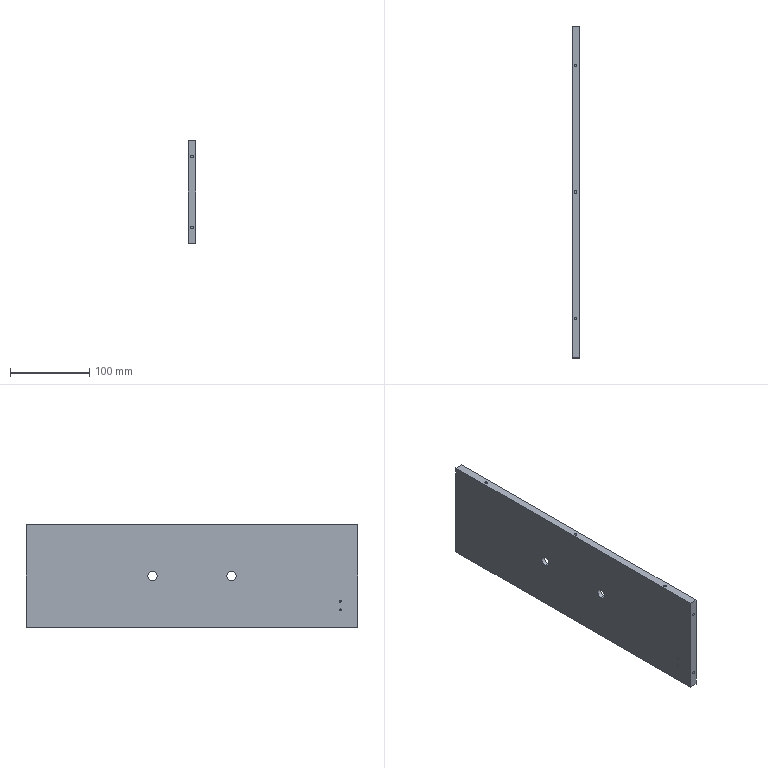Part | SolidWorks | features BaseBody 1 | 1 solid | 48 faces | box 10 x 420 x 130 mm | volume 527833 mm3 | cylinder 31 | plane 13 | cone 4 | commonest cylinder face diameters 3.3 x19 2.5 x4 12 x4 45 x4
STEP:
#1=CARTESIAN_POINT('',(-903.891,738.647,281.732));
#2=VERTEX_POINT('',#1);
#3=CARTESIAN_POINT('',(-905.541,740.297,281.732));
#4=VERTEX_POINT('',#3);
#5=CARTESIAN_POINT('',(-903.891,740.297,281.732));
#6=DIRECTION('',(0.,0.,-1.));
#7=DIRECTION('',(-1.,0.,0.));
#8=AXIS2_PLACEMENT_3D('',#5,#6,#7);
#9=CIRCLE('',#8,1.65);
#10=EDGE_CURVE('',#2,#4,#9,.T.);
#11=ORIENTED_EDGE('',*,*,#10,.T.);
#12=CARTESIAN_POINT('',(-905.541,740.297,301.732));
#13=VERTEX_POINT('',#12);
#14=CARTESIAN_POINT('',(-905.541,740.297,301.732));
#15=DIRECTION('',(0.,0.,1.));
#16=VECTOR('',#15,1000.);
#17=LINE('',#14,#16);
#18=EDGE_CURVE('',#4,#13,#17,.T.);
#19=ORIENTED_EDGE('',*,*,#18,.T.);
#20=CARTESIAN_POINT('',(-903.891,738.647,301.732));
#21=VERTEX_POINT('',#20);
#22=CARTESIAN_POINT('',(-903.891,740.297,301.732));
#23=DIRECTION('',(0.,0.,1.));
#24=DIRECTION('',(-1.,0.,0.));
#25=AXIS2_PLACEMENT_3D('',#22,#23,#24);
#26=CIRCLE('',#25,1.65);
#27=EDGE_CURVE('',#13,#21,#26,.T.);
#28=ORIENTED_EDGE('',*,*,#27,.T.);
#29=CARTESIAN_POINT('',(-903.891,738.647,301.732));
#30=DIRECTION('',(0.,0.,-1.));
#31=VECTOR('',#30,1000.);
#32=LINE('',#29,#31);
#33=EDGE_CURVE('',#21,#2,#32,.T.);
#34=ORIENTED_EDGE('',*,*,#33,.T.);
#35=EDGE_LOOP('',(#11,#19,#28,#34));
#36=FACE_OUTER_BOUND('',#35,.T.);
#37=CARTESIAN_POINT('',(-903.891,740.297,301.732));
#38=DIRECTION('',(0.,0.,1.));
#39=DIRECTION('',(-1.,0.,0.));
#40=AXIS2_PLACEMENT_3D('',#37,#38,#39);
#41=CYLINDRICAL_SURFACE('',#40,1.65);
#42=ADVANCED_FACE('',(#36),#41,.F.);
#43=CARTESIAN_POINT('',(-903.891,578.647,281.732));
#44=VERTEX_POINT('',#43);
#45=CARTESIAN_POINT('',(-905.541,580.297,281.732));
#46=VERTEX_POINT('',#45);
#47=CARTESIAN_POINT('',(-903.891,580.297,281.732));
#48=DIRECTION('',(0.,0.,-1.));
#49=DIRECTION('',(-1.,0.,0.));
#50=AXIS2_PLACEMENT_3D('',#47,#48,#49);
#51=CIRCLE('',#50,1.65);
#52=EDGE_CURVE('',#44,#46,#51,.T.);
#53=ORIENTED_EDGE('',*,*,#52,.T.);
#54=CARTESIAN_POINT('',(-905.541,580.297,301.732));
#55=VERTEX_POINT('',#54);
#56=CARTESIAN_POINT('',(-905.541,580.297,301.732));
#57=DIRECTION('',(0.,0.,1.));
#58=VECTOR('',#57,1000.);
#59=LINE('',#56,#58);
#60=EDGE_CURVE('',#46,#55,#59,.T.);
#61=ORIENTED_EDGE('',*,*,#60,.T.);
#62=CARTESIAN_POINT('',(-903.891,578.647,301.732));
#63=VERTEX_POINT('',#62);
#64=CARTESIAN_POINT('',(-903.891,580.297,301.732));
#65=DIRECTION('',(0.,0.,1.));
#66=DIRECTION('',(-1.,0.,0.));
#67=AXIS2_PLACEMENT_3D('',#64,#65,#66);
#68=CIRCLE('',#67,1.65);
#69=EDGE_CURVE('',#55,#63,#68,.T.);
#70=ORIENTED_EDGE('',*,*,#69,.T.);
#71=CARTESIAN_POINT('',(-903.891,578.647,301.732));
#72=DIRECTION('',(0.,0.,-1.));
#73=VECTOR('',#72,1000.);
#74=LINE('',#71,#73);
#75=EDGE_CURVE('',#63,#44,#74,.T.);
#76=ORIENTED_EDGE('',*,*,#75,.T.);
#77=EDGE_LOOP('',(#53,#61,#70,#76));
#78=FACE_OUTER_BOUND('',#77,.T.);
#79=CARTESIAN_POINT('',(-903.891,580.297,301.732));
#80=DIRECTION('',(0.,0.,1.));
#81=DIRECTION('',(-1.,0.,0.));
#82=AXIS2_PLACEMENT_3D('',#79,#80,#81);
#83=CYLINDRICAL_SURFACE('',#82,1.65);
#84=ADVANCED_FACE('',(#78),#83,.F.);
#85=CARTESIAN_POINT('',(-903.891,418.647,281.732));
#86=VERTEX_POINT('',#85);
#87=CARTESIAN_POINT('',(-905.541,420.297,281.732));
#88=VERTEX_POINT('',#87);
#89=CARTESIAN_POINT('',(-903.891,420.297,281.732));
#90=DIRECTION('',(0.,0.,-1.));
#91=DIRECTION('',(-1.,0.,0.));
#92=AXIS2_PLACEMENT_3D('',#89,#90,#91);
#93=CIRCLE('',#92,1.65);
#94=EDGE_CURVE('',#86,#88,#93,.T.);
#95=ORIENTED_EDGE('',*,*,#94,.T.);
#96=CARTESIAN_POINT('',(-905.541,420.297,301.732));
#97=VERTEX_POINT('',#96);
#98=CARTESIAN_POINT('',(-905.541,420.297,301.732));
#99=DIRECTION('',(0.,0.,1.));
#100=VECTOR('',#99,1000.);
#101=LINE('',#98,#100);
#102=EDGE_CURVE('',#88,#97,#101,.T.);
#103=ORIENTED_EDGE('',*,*,#102,.T.);
#104=CARTESIAN_POINT('',(-903.891,418.647,301.732));
#105=VERTEX_POINT('',#104);
#106=CARTESIAN_POINT('',(-903.891,420.297,301.732));
#107=DIRECTION('',(0.,0.,1.));
#108=DIRECTION('',(-1.,0.,0.));
#109=AXIS2_PLACEMENT_3D('',#106,#107,#108);
#110=CIRCLE('',#109,1.65);
#111=EDGE_CURVE('',#97,#105,#110,.T.);
#112=ORIENTED_EDGE('',*,*,#111,.T.);
#113=CARTESIAN_POINT('',(-903.891,418.647,301.732));
#114=DIRECTION('',(0.,0.,-1.));
#115=VECTOR('',#114,1000.);
#116=LINE('',#113,#115);
#117=EDGE_CURVE('',#105,#86,#116,.T.);
#118=ORIENTED_EDGE('',*,*,#117,.T.);
#119=EDGE_LOOP('',(#95,#103,#112,#118));
#120=FACE_OUTER_BOUND('',#119,.T.);
#121=CARTESIAN_POINT('',(-903.891,420.297,301.732));
#122=DIRECTION('',(0.,0.,1.));
#123=DIRECTION('',(-1.,0.,0.));
#124=AXIS2_PLACEMENT_3D('',#121,#122,#123);
#125=CYLINDRICAL_SURFACE('',#124,1.65);
#126=ADVANCED_FACE('',(#120),#125,.F.);
#127=CARTESIAN_POINT('',(-903.131,390.297,283.382));
#128=VERTEX_POINT('',#127);
#129=CARTESIAN_POINT('',(-901.481,390.297,281.732));
#130=VERTEX_POINT('',#129);
#131=CARTESIAN_POINT('',(-903.131,390.297,281.732));
#132=DIRECTION('',(0.,1.,0.));
#133=DIRECTION('',(1.,0.,0.));
#134=AXIS2_PLACEMENT_3D('',#131,#132,#133);
#135=CIRCLE('',#134,1.65);
#136=EDGE_CURVE('',#128,#130,#135,.T.);
#137=ORIENTED_EDGE('',*,*,#136,.T.);
#138=CARTESIAN_POINT('',(-901.481,370.297,281.732));
#139=VERTEX_POINT('',#138);
#140=CARTESIAN_POINT('',(-901.481,370.297,281.732));
#141=DIRECTION('',(0.,-1.,0.));
#142=VECTOR('',#141,1000.);
#143=LINE('',#140,#142);
#144=EDGE_CURVE('',#130,#139,#143,.T.);
#145=ORIENTED_EDGE('',*,*,#144,.T.);
#146=CARTESIAN_POINT('',(-903.131,370.297,283.382));
#147=VERTEX_POINT('',#146);
#148=CARTESIAN_POINT('',(-903.131,370.297,281.732));
#149=DIRECTION('',(0.,-1.,0.));
#150=DIRECTION('',(0.,0.,-1.));
#151=AXIS2_PLACEMENT_3D('',#148,#149,#150);
#152=CIRCLE('',#151,1.65);
#153=EDGE_CURVE('',#139,#147,#152,.T.);
#154=ORIENTED_EDGE('',*,*,#153,.T.);
#155=CARTESIAN_POINT('',(-903.131,390.297,283.382));
#156=DIRECTION('',(0.,-1.,0.));
#157=VECTOR('',#156,1000.);
#158=LINE('',#155,#157);
#159=EDGE_CURVE('',#128,#147,#158,.T.);
#160=ORIENTED_EDGE('',*,*,#159,.F.);
#161=EDGE_LOOP('',(#137,#145,#154,#160));
#162=FACE_OUTER_BOUND('',#161,.T.);
#163=CARTESIAN_POINT('',(-903.131,370.297,281.732));
#164=DIRECTION('',(0.,-1.,0.));
#165=DIRECTION('',(1.,0.,0.));
#166=AXIS2_PLACEMENT_3D('',#163,#164,#165);
#167=CYLINDRICAL_SURFACE('',#166,1.65);
#168=ADVANCED_FACE('',(#162),#167,.F.);
#169=CARTESIAN_POINT('',(-903.131,390.297,193.382));
#170=VERTEX_POINT('',#169);
#171=CARTESIAN_POINT('',(-901.481,390.297,191.732));
#172=VERTEX_POINT('',#171);
#173=CARTESIAN_POINT('',(-903.131,390.297,191.732));
#174=DIRECTION('',(0.,1.,0.));
#175=DIRECTION('',(1.,0.,0.));
#176=AXIS2_PLACEMENT_3D('',#173,#174,#175);
#177=CIRCLE('',#176,1.65);
#178=EDGE_CURVE('',#170,#172,#177,.T.);
#179=ORIENTED_EDGE('',*,*,#178,.T.);
#180=CARTESIAN_POINT('',(-901.481,370.297,191.732));
#181=VERTEX_POINT('',#180);
#182=CARTESIAN_POINT('',(-901.481,370.297,191.732));
#183=DIRECTION('',(0.,-1.,0.));
#184=VECTOR('',#183,1000.);
#185=LINE('',#182,#184);
#186=EDGE_CURVE('',#172,#181,#185,.T.);
#187=ORIENTED_EDGE('',*,*,#186,.T.);
#188=CARTESIAN_POINT('',(-903.131,370.297,193.382));
#189=VERTEX_POINT('',#188);
#190=CARTESIAN_POINT('',(-903.131,370.297,191.732));
#191=DIRECTION('',(0.,-1.,0.));
#192=DIRECTION('',(0.,0.,-1.));
#193=AXIS2_PLACEMENT_3D('',#190,#191,#192);
#194=CIRCLE('',#193,1.65);
#195=EDGE_CURVE('',#181,#189,#194,.T.);
#196=ORIENTED_EDGE('',*,*,#195,.T.);
#197=CARTESIAN_POINT('',(-903.131,390.297,193.382));
#198=DIRECTION('',(0.,-1.,0.));
#199=VECTOR('',#198,1000.);
#200=LINE('',#197,#199);
#201=EDGE_CURVE('',#170,#189,#200,.T.);
#202=ORIENTED_EDGE('',*,*,#201,.F.);
#203=EDGE_LOOP('',(#179,#187,#196,#202));
#204=FACE_OUTER_BOUND('',#203,.T.);
#205=CARTESIAN_POINT('',(-903.131,370.297,191.732));
#206=DIRECTION('',(0.,-1.,0.));
#207=DIRECTION('',(1.,0.,0.));
#208=AXIS2_PLACEMENT_3D('',#205,#206,#207);
#209=CYLINDRICAL_SURFACE('',#208,1.65);
#210=ADVANCED_FACE('',(#204),#209,.F.);
#211=CARTESIAN_POINT('',(-904.781,790.297,191.732));
#212=VERTEX_POINT('',#211);
#213=CARTESIAN_POINT('',(-901.481,790.297,191.732));
#214=VERTEX_POINT('',#213);
#215=CARTESIAN_POINT('',(-903.131,790.297,191.732));
#216=DIRECTION('',(0.,1.,0.));
#217=DIRECTION('',(-1.,0.,0.));
#218=AXIS2_PLACEMENT_3D('',#215,#216,#217);
#219=CIRCLE('',#218,1.65);
#220=EDGE_CURVE('',#212,#214,#219,.T.);
#221=ORIENTED_EDGE('',*,*,#220,.T.);
#222=CARTESIAN_POINT('',(-901.481,780.197,191.732));
#223=VERTEX_POINT('',#222);
#224=CARTESIAN_POINT('',(-901.481,780.197,191.732));
#225=DIRECTION('',(0.,1.,0.));
#226=VECTOR('',#225,1000.);
#227=LINE('',#224,#226);
#228=EDGE_CURVE('',#223,#214,#227,.T.);
#229=ORIENTED_EDGE('',*,*,#228,.F.);
#230=CARTESIAN_POINT('',(-904.781,780.197,191.732));
#231=VERTEX_POINT('',#230);
#232=CARTESIAN_POINT('',(-903.131,780.197,191.732));
#233=DIRECTION('',(0.,-1.,0.));
#234=DIRECTION('',(1.,0.,0.));
#235=AXIS2_PLACEMENT_3D('',#232,#233,#234);
#236=CIRCLE('',#235,1.65);
#237=EDGE_CURVE('',#223,#231,#236,.T.);
#238=ORIENTED_EDGE('',*,*,#237,.T.);
#239=CARTESIAN_POINT('',(-904.781,790.297,191.732));
#240=DIRECTION('',(0.,-1.,0.));
#241=VECTOR('',#240,1000.);
#242=LINE('',#239,#241);
#243=EDGE_CURVE('',#212,#231,#242,.T.);
#244=ORIENTED_EDGE('',*,*,#243,.F.);
#245=EDGE_LOOP('',(#221,#229,#238,#244));
#246=FACE_OUTER_BOUND('',#245,.T.);
#247=CARTESIAN_POINT('',(-903.131,790.297,191.732));
#248=DIRECTION('',(0.,1.,0.));
#249=DIRECTION('',(-1.,0.,0.));
#250=AXIS2_PLACEMENT_3D('',#247,#248,#249);
#251=CYLINDRICAL_SURFACE('',#250,1.65);
#252=ADVANCED_FACE('',(#246),#251,.F.);
#253=ORIENTED_EDGE('',*,*,#228,.T.);
#254=CARTESIAN_POINT('',(-903.131,790.297,191.732));
#255=DIRECTION('',(0.,1.,0.));
#256=DIRECTION('',(1.,0.,0.));
#257=AXIS2_PLACEMENT_3D('',#254,#255,#256);
#258=CIRCLE('',#257,1.65);
#259=EDGE_CURVE('',#214,#212,#258,.T.);
#260=ORIENTED_EDGE('',*,*,#259,.T.);
#261=ORIENTED_EDGE('',*,*,#243,.T.);
#262=CARTESIAN_POINT('',(-903.131,780.197,191.732));
#263=DIRECTION('',(0.,-1.,0.));
#264=DIRECTION('',(-1.,0.,0.));
#265=AXIS2_PLACEMENT_3D('',#262,#263,#264);
#266=CIRCLE('',#265,1.65);
#267=EDGE_CURVE('',#231,#223,#266,.T.);
#268=ORIENTED_EDGE('',*,*,#267,.T.);
#269=EDGE_LOOP('',(#253,#260,#261,#268));
#270=FACE_OUTER_BOUND('',#269,.T.);
#271=CARTESIAN_POINT('',(-903.131,790.297,191.732));
#272=DIRECTION('',(0.,1.,0.));
#273=DIRECTION('',(-1.,0.,0.));
#274=AXIS2_PLACEMENT_3D('',#271,#272,#273);
#275=CYLINDRICAL_SURFACE('',#274,1.65);
#276=ADVANCED_FACE('',(#270),#275,.F.);
#277=ORIENTED_EDGE('',*,*,#267,.F.);
#278=CARTESIAN_POINT('',(-903.131,779.205,191.732));
#279=VERTEX_POINT('',#278);
#280=CARTESIAN_POINT('',(-904.781,780.197,191.732));
#281=DIRECTION('',(0.8572,-0.515,0.));
#282=VECTOR('',#281,1000.);
#283=LINE('',#280,#282);
#284=EDGE_CURVE('',#231,#279,#283,.T.);
#285=ORIENTED_EDGE('',*,*,#284,.T.);
#286=CARTESIAN_POINT('',(-903.131,779.205,191.732));
#287=DIRECTION('',(0.8572,0.515,0.));
#288=VECTOR('',#287,1000.);
#289=LINE('',#286,#288);
#290=EDGE_CURVE('',#279,#223,#289,.T.);
#291=ORIENTED_EDGE('',*,*,#290,.T.);
#292=EDGE_LOOP('',(#277,#285,#291));
#293=FACE_OUTER_BOUND('',#292,.T.);
#294=CARTESIAN_POINT('',(-903.131,779.837,191.732));
#295=DIRECTION('',(0.,1.,0.));
#296=DIRECTION('',(1.,0.,0.));
#297=AXIS2_PLACEMENT_3D('',#294,#295,#296);
#298=CONICAL_SURFACE('',#297,1.051,1.03);
#299=ADVANCED_FACE('',(#293),#298,.F.);
#300=ORIENTED_EDGE('',*,*,#237,.F.);
#301=ORIENTED_EDGE('',*,*,#290,.F.);
#302=ORIENTED_EDGE('',*,*,#284,.F.);
#303=EDGE_LOOP('',(#300,#301,#302));
#304=FACE_OUTER_BOUND('',#303,.T.);
#305=CARTESIAN_POINT('',(-903.131,779.837,191.732));
#306=DIRECTION('',(0.,1.,0.));
#307=DIRECTION('',(1.,0.,0.));
#308=AXIS2_PLACEMENT_3D('',#305,#306,#307);
#309=CONICAL_SURFACE('',#308,1.051,1.03);
#310=ADVANCED_FACE('',(#304),#309,.F.);
#311=CARTESIAN_POINT('',(-898.131,790.297,171.732));
#312=VERTEX_POINT('',#311);
#313=CARTESIAN_POINT('',(-898.131,790.297,301.732));
#314=VERTEX_POINT('',#313);
#315=CARTESIAN_POINT('',(-898.131,790.297,171.732));
#316=DIRECTION('',(0.,0.,1.));
#317=VECTOR('',#316,1000.);
#318=LINE('',#315,#317);
#319=EDGE_CURVE('',#312,#314,#318,.T.);
#320=ORIENTED_EDGE('',*,*,#319,.F.);
#321=CARTESIAN_POINT('',(-908.131,790.297,171.732));
#322=VERTEX_POINT('',#321);
#323=CARTESIAN_POINT('',(-908.131,790.297,171.732));
#324=DIRECTION('',(1.,0.,0.));
#325=VECTOR('',#324,1000.);
#326=LINE('',#323,#325);
#327=EDGE_CURVE('',#322,#312,#326,.T.);
#328=ORIENTED_EDGE('',*,*,#327,.F.);
#329=CARTESIAN_POINT('',(-908.131,790.297,301.732));
#330=VERTEX_POINT('',#329);
#331=CARTESIAN_POINT('',(-908.131,790.297,301.732));
#332=DIRECTION('',(0.,0.,-1.));
#333=VECTOR('',#332,1000.);
#334=LINE('',#331,#333);
#335=EDGE_CURVE('',#330,#322,#334,.T.);
#336=ORIENTED_EDGE('',*,*,#335,.F.);
#337=CARTESIAN_POINT('',(-898.131,790.297,301.732));
#338=DIRECTION('',(-1.,0.,0.));
#339=VECTOR('',#338,1000.);
#340=LINE('',#337,#339);
#341=EDGE_CURVE('',#314,#330,#340,.T.);
#342=ORIENTED_EDGE('',*,*,#341,.F.);
#343=EDGE_LOOP('',(#320,#328,#336,#342));
#344=FACE_OUTER_BOUND('',#343,.T.);
#345=CARTESIAN_POINT('',(-901.481,790.297,281.732));
#346=VERTEX_POINT('',#345);
#347=CARTESIAN_POINT('',(-904.781,790.297,281.732));
#348=VERTEX_POINT('',#347);
#349=CARTESIAN_POINT('',(-903.131,790.297,281.732));
#350=DIRECTION('',(0.,1.,0.));
#351=DIRECTION('',(1.,0.,0.));
#352=AXIS2_PLACEMENT_3D('',#349,#350,#351);
#353=CIRCLE('',#352,1.65);
#354=EDGE_CURVE('',#346,#348,#353,.T.);
#355=ORIENTED_EDGE('',*,*,#354,.F.);
#356=CARTESIAN_POINT('',(-903.131,790.297,281.732));
#357=DIRECTION('',(0.,1.,0.));
#358=DIRECTION('',(-1.,0.,0.));
#359=AXIS2_PLACEMENT_3D('',#356,#357,#358);
#360=CIRCLE('',#359,1.65);
#361=EDGE_CURVE('',#348,#346,#360,.T.);
#362=ORIENTED_EDGE('',*,*,#361,.F.);
#363=EDGE_LOOP('',(#355,#362));
#364=FACE_BOUND('',#363,.T.);
#365=ORIENTED_EDGE('',*,*,#259,.F.);
#366=ORIENTED_EDGE('',*,*,#220,.F.);
#367=EDGE_LOOP('',(#365,#366));
#368=FACE_BOUND('',#367,.T.);
#369=CARTESIAN_POINT('',(-898.131,790.297,301.732));
#370=DIRECTION('',(0.,-1.,0.));
#371=DIRECTION('',(1.,0.,0.));
#372=AXIS2_PLACEMENT_3D('',#369,#370,#371);
#373=PLANE('',#372);
#374=ADVANCED_FACE('',(#344,#364,#368),#373,.F.);
#375=CARTESIAN_POINT('',(-898.131,370.297,301.732));
#376=VERTEX_POINT('',#375);
#377=CARTESIAN_POINT('',(-898.131,790.297,301.732));
#378=DIRECTION('',(0.,-1.,0.));
#379=VECTOR('',#378,1000.);
#380=LINE('',#377,#379);
#381=EDGE_CURVE('',#314,#376,#380,.T.);
#382=ORIENTED_EDGE('',*,*,#381,.F.);
#383=ORIENTED_EDGE('',*,*,#341,.T.);
#384=CARTESIAN_POINT('',(-908.131,370.297,301.732));
#385=VERTEX_POINT('',#384);
#386=CARTESIAN_POINT('',(-908.131,790.297,301.732));
#387=DIRECTION('',(0.,-1.,0.));
#388=VECTOR('',#387,1000.);
#389=LINE('',#386,#388);
#390=EDGE_CURVE('',#330,#385,#389,.T.);
#391=ORIENTED_EDGE('',*,*,#390,.T.);
#392=CARTESIAN_POINT('',(-908.131,370.297,301.732));
#393=DIRECTION('',(1.,0.,0.));
#394=VECTOR('',#393,1000.);
#395=LINE('',#392,#394);
#396=EDGE_CURVE('',#385,#376,#395,.T.);
#397=ORIENTED_EDGE('',*,*,#396,.T.);
#398=EDGE_LOOP('',(#382,#383,#391,#397));
#399=FACE_OUTER_BOUND('',#398,.T.);
#400=CARTESIAN_POINT('',(-903.891,421.947,301.732));
#401=VERTEX_POINT('',#400);
#402=CARTESIAN_POINT('',(-903.891,420.297,301.732));
#403=DIRECTION('',(0.,0.,1.));
#404=DIRECTION('',(-1.,0.,0.));
#405=AXIS2_PLACEMENT_3D('',#402,#403,#404);
#406=CIRCLE('',#405,1.65);
#407=EDGE_CURVE('',#401,#97,#406,.T.);
#408=ORIENTED_EDGE('',*,*,#407,.F.);
#409=CARTESIAN_POINT('',(-903.891,420.297,301.732));
#410=DIRECTION('',(0.,0.,1.));
#411=DIRECTION('',(0.,-1.,0.));
#412=AXIS2_PLACEMENT_3D('',#409,#410,#411);
#413=CIRCLE('',#412,1.65);
#414=EDGE_CURVE('',#105,#401,#413,.T.);
#415=ORIENTED_EDGE('',*,*,#414,.F.);
#416=ORIENTED_EDGE('',*,*,#111,.F.);
#417=EDGE_LOOP('',(#408,#415,#416));
#418=FACE_BOUND('',#417,.T.);
#419=CARTESIAN_POINT('',(-903.891,581.947,301.732));
#420=VERTEX_POINT('',#419);
#421=CARTESIAN_POINT('',(-903.891,580.297,301.732));
#422=DIRECTION('',(0.,0.,1.));
#423=DIRECTION('',(-1.,0.,0.));
#424=AXIS2_PLACEMENT_3D('',#421,#422,#423);
#425=CIRCLE('',#424,1.65);
#426=EDGE_CURVE('',#420,#55,#425,.T.);
#427=ORIENTED_EDGE('',*,*,#426,.F.);
#428=CARTESIAN_POINT('',(-903.891,580.297,301.732));
#429=DIRECTION('',(0.,0.,1.));
#430=DIRECTION('',(0.,-1.,0.));
#431=AXIS2_PLACEMENT_3D('',#428,#429,#430);
#432=CIRCLE('',#431,1.65);
#433=EDGE_CURVE('',#63,#420,#432,.T.);
#434=ORIENTED_EDGE('',*,*,#433,.F.);
#435=ORIENTED_EDGE('',*,*,#69,.F.);
#436=EDGE_LOOP('',(#427,#434,#435));
#437=FACE_BOUND('',#436,.T.);
#438=CARTESIAN_POINT('',(-903.891,741.947,301.732));
#439=VERTEX_POINT('',#438);
#440=CARTESIAN_POINT('',(-903.891,740.297,301.732));
#441=DIRECTION('',(0.,0.,1.));
#442=DIRECTION('',(-1.,0.,0.));
#443=AXIS2_PLACEMENT_3D('',#440,#441,#442);
#444=CIRCLE('',#443,1.65);
#445=EDGE_CURVE('',#439,#13,#444,.T.);
#446=ORIENTED_EDGE('',*,*,#445,.F.);
#447=CARTESIAN_POINT('',(-903.891,740.297,301.732));
#448=DIRECTION('',(0.,0.,1.));
#449=DIRECTION('',(0.,-1.,0.));
#450=AXIS2_PLACEMENT_3D('',#447,#448,#449);
#451=CIRCLE('',#450,1.65);
#452=EDGE_CURVE('',#21,#439,#451,.T.);
#453=ORIENTED_EDGE('',*,*,#452,.F.);
#454=ORIENTED_EDGE('',*,*,#27,.F.);
#455=EDGE_LOOP('',(#446,#453,#454));
#456=FACE_BOUND('',#455,.T.);
#457=CARTESIAN_POINT('',(-898.131,790.297,301.732));
#458=DIRECTION('',(0.,0.,-1.));
#459=DIRECTION('',(0.,-1.,0.));
#460=AXIS2_PLACEMENT_3D('',#457,#458,#459);
#461=PLANE('',#460);
#462=ADVANCED_FACE('',(#399,#418,#437,#456),#461,.F.);
#463=CARTESIAN_POINT('',(-898.131,370.297,171.732));
#464=VERTEX_POINT('',#463);
#465=CARTESIAN_POINT('',(-898.131,370.297,301.732));
#466=DIRECTION('',(0.,0.,-1.));
#467=VECTOR('',#466,1000.);
#468=LINE('',#465,#467);
#469=EDGE_CURVE('',#376,#464,#468,.T.);
#470=ORIENTED_EDGE('',*,*,#469,.F.);
#471=ORIENTED_EDGE('',*,*,#396,.F.);
#472=CARTESIAN_POINT('',(-908.131,370.297,171.732));
#473=VERTEX_POINT('',#472);
#474=CARTESIAN_POINT('',(-908.131,370.297,301.732));
#475=DIRECTION('',(0.,0.,-1.));
#476=VECTOR('',#475,1000.);
#477=LINE('',#474,#476);
#478=EDGE_CURVE('',#385,#473,#477,.T.);
#479=ORIENTED_EDGE('',*,*,#478,.T.);
#480=CARTESIAN_POINT('',(-908.131,370.297,171.732));
#481=DIRECTION('',(1.,0.,0.));
#482=VECTOR('',#481,1000.);
#483=LINE('',#480,#482);
#484=EDGE_CURVE('',#473,#464,#483,.T.);
#485=ORIENTED_EDGE('',*,*,#484,.T.);
#486=EDGE_LOOP('',(#470,#471,#479,#485));
#487=FACE_OUTER_BOUND('',#486,.T.);
#488=CARTESIAN_POINT('',(-903.131,370.297,190.082));
#489=VERTEX_POINT('',#488);
#490=CARTESIAN_POINT('',(-903.131,370.297,191.732));
#491=DIRECTION('',(0.,-1.,0.));
#492=DIRECTION('',(-1.,0.,0.));
#493=AXIS2_PLACEMENT_3D('',#490,#491,#492);
#494=CIRCLE('',#493,1.65);
#495=EDGE_CURVE('',#189,#489,#494,.T.);
#496=ORIENTED_EDGE('',*,*,#495,.F.);
#497=ORIENTED_EDGE('',*,*,#195,.F.);
#498=CARTESIAN_POINT('',(-903.131,370.297,191.732));
#499=DIRECTION('',(0.,-1.,0.));
#500=DIRECTION('',(0.,0.,-1.));
#501=AXIS2_PLACEMENT_3D('',#498,#499,#500);
#502=CIRCLE('',#501,1.65);
#503=EDGE_CURVE('',#489,#181,#502,.T.);
#504=ORIENTED_EDGE('',*,*,#503,.F.);
#505=EDGE_LOOP('',(#496,#497,#504));
#506=FACE_BOUND('',#505,.T.);
#507=CARTESIAN_POINT('',(-903.131,370.297,280.082));
#508=VERTEX_POINT('',#507);
#509=CARTESIAN_POINT('',(-903.131,370.297,281.732));
#510=DIRECTION('',(0.,-1.,0.));
#511=DIRECTION('',(-1.,0.,0.));
#512=AXIS2_PLACEMENT_3D('',#509,#510,#511);
#513=CIRCLE('',#512,1.65);
#514=EDGE_CURVE('',#147,#508,#513,.T.);
#515=ORIENTED_EDGE('',*,*,#514,.F.);
#516=ORIENTED_EDGE('',*,*,#153,.F.);
#517=CARTESIAN_POINT('',(-903.131,370.297,281.732));
#518=DIRECTION('',(0.,-1.,0.));
#519=DIRECTION('',(0.,0.,-1.));
#520=AXIS2_PLACEMENT_3D('',#517,#518,#519);
#521=CIRCLE('',#520,1.65);
#522=EDGE_CURVE('',#508,#139,#521,.T.);
#523=ORIENTED_EDGE('',*,*,#522,.F.);
#524=EDGE_LOOP('',(#515,#516,#523));
#525=FACE_BOUND('',#524,.T.);
#526=CARTESIAN_POINT('',(-898.131,370.297,301.732));
#527=DIRECTION('',(0.,1.,0.));
#528=DIRECTION('',(-1.,0.,0.));
#529=AXIS2_PLACEMENT_3D('',#526,#527,#528);
#530=PLANE('',#529);
#531=ADVANCED_FACE('',(#487,#506,#525),#530,.F.);
#532=CARTESIAN_POINT('',(-898.131,370.297,171.732));
#533=DIRECTION('',(0.,1.,0.));
#534=VECTOR('',#533,1000.);
#535=LINE('',#532,#534);
#536=EDGE_CURVE('',#464,#312,#535,.T.);
#537=ORIENTED_EDGE('',*,*,#536,.F.);
#538=ORIENTED_EDGE('',*,*,#484,.F.);
#539=CARTESIAN_POINT('',(-908.131,370.297,171.732));
#540=DIRECTION('',(0.,1.,0.));
#541=VECTOR('',#540,1000.);
#542=LINE('',#539,#541);
#543=EDGE_CURVE('',#473,#322,#542,.T.);
#544=ORIENTED_EDGE('',*,*,#543,.T.);
#545=ORIENTED_EDGE('',*,*,#327,.T.);
#546=EDGE_LOOP('',(#537,#538,#544,#545));
#547=FACE_OUTER_BOUND('',#546,.T.);
#548=CARTESIAN_POINT('',(-898.131,790.297,171.732));
#549=DIRECTION('',(0.,0.,1.));
#550=DIRECTION('',(0.,1.,0.));
#551=AXIS2_PLACEMENT_3D('',#548,#549,#550);
#552=PLANE('',#551);
#553=ADVANCED_FACE('',(#547),#552,.F.);
#554=ORIENTED_EDGE('',*,*,#390,.F.);
#555=ORIENTED_EDGE('',*,*,#335,.T.);
#556=ORIENTED_EDGE('',*,*,#543,.F.);
#557=ORIENTED_EDGE('',*,*,#478,.F.);
#558=EDGE_LOOP('',(#554,#555,#556,#557));
#559=FACE_OUTER_BOUND('',#558,.T.);
#560=CARTESIAN_POINT('',(-908.131,392.797,194.982));
#561=VERTEX_POINT('',#560);
#562=CARTESIAN_POINT('',(-908.131,392.797,192.482));
#563=VERTEX_POINT('',#562);
#564=CARTESIAN_POINT('',(-908.131,392.797,193.732));
#565=DIRECTION('',(-1.,0.,0.));
#566=DIRECTION('',(0.,0.,1.));
#567=AXIS2_PLACEMENT_3D('',#564,#565,#566);
#568=CIRCLE('',#567,1.25);
#569=EDGE_CURVE('',#561,#563,#568,.T.);
#570=ORIENTED_EDGE('',*,*,#569,.F.);
#571=CARTESIAN_POINT('',(-908.131,392.797,193.732));
#572=DIRECTION('',(-1.,0.,0.));
#573=DIRECTION('',(0.,0.,-1.));
#574=AXIS2_PLACEMENT_3D('',#571,#572,#573);
#575=CIRCLE('',#574,1.25);
#576=EDGE_CURVE('',#563,#561,#575,.T.);
#577=ORIENTED_EDGE('',*,*,#576,.F.);
#578=EDGE_LOOP('',(#570,#577));
#579=FACE_BOUND('',#578,.T.);
#580=CARTESIAN_POINT('',(-908.131,392.797,205.982));
#581=VERTEX_POINT('',#580);
#582=CARTESIAN_POINT('',(-908.131,392.797,203.482));
#583=VERTEX_POINT('',#582);
#584=CARTESIAN_POINT('',(-908.131,392.797,204.732));
#585=DIRECTION('',(-1.,0.,0.));
#586=DIRECTION('',(0.,0.,1.));
#587=AXIS2_PLACEMENT_3D('',#584,#585,#586);
#588=CIRCLE('',#587,1.25);
#589=EDGE_CURVE('',#581,#583,#588,.T.);
#590=ORIENTED_EDGE('',*,*,#589,.F.);
#591=CARTESIAN_POINT('',(-908.131,392.797,204.732));
#592=DIRECTION('',(-1.,0.,0.));
#593=DIRECTION('',(0.,0.,-1.));
#594=AXIS2_PLACEMENT_3D('',#591,#592,#593);
#595=CIRCLE('',#594,1.25);
#596=EDGE_CURVE('',#583,#581,#595,.T.);
#597=ORIENTED_EDGE('',*,*,#596,.F.);
#598=EDGE_LOOP('',(#590,#597));
#599=FACE_BOUND('',#598,.T.);
#600=CARTESIAN_POINT('',(-908.131,530.297,242.732));
#601=VERTEX_POINT('',#600);
#602=CARTESIAN_POINT('',(-908.131,530.297,230.732));
#603=VERTEX_POINT('',#602);
#604=CARTESIAN_POINT('',(-908.131,530.297,236.732));
#605=DIRECTION('',(-1.,0.,0.));
#606=DIRECTION('',(0.,0.,1.));
#607=AXIS2_PLACEMENT_3D('',#604,#605,#606);
#608=CIRCLE('',#607,6.);
#609=EDGE_CURVE('',#601,#603,#608,.T.);
#610=ORIENTED_EDGE('',*,*,#609,.F.);
#611=CARTESIAN_POINT('',(-908.131,530.297,236.732));
#612=DIRECTION('',(-1.,0.,0.));
#613=DIRECTION('',(0.,0.,-1.));
#614=AXIS2_PLACEMENT_3D('',#611,#612,#613);
#615=CIRCLE('',#614,6.);
#616=EDGE_CURVE('',#603,#601,#615,.T.);
#617=ORIENTED_EDGE('',*,*,#616,.F.);
#618=EDGE_LOOP('',(#610,#617));
#619=FACE_BOUND('',#618,.T.);
#620=CARTESIAN_POINT('',(-908.131,630.297,242.732));
#621=VERTEX_POINT('',#620);
#622=CARTESIAN_POINT('',(-908.131,630.297,230.732));
#623=VERTEX_POINT('',#622);
#624=CARTESIAN_POINT('',(-908.131,630.297,236.732));
#625=DIRECTION('',(-1.,0.,0.));
#626=DIRECTION('',(0.,0.,1.));
#627=AXIS2_PLACEMENT_3D('',#624,#625,#626);
#628=CIRCLE('',#627,6.);
#629=EDGE_CURVE('',#621,#623,#628,.T.);
#630=ORIENTED_EDGE('',*,*,#629,.F.);
#631=CARTESIAN_POINT('',(-908.131,630.297,236.732));
#632=DIRECTION('',(-1.,0.,0.));
#633=DIRECTION('',(0.,0.,-1.));
#634=AXIS2_PLACEMENT_3D('',#631,#632,#633);
#635=CIRCLE('',#634,6.);
#636=EDGE_CURVE('',#623,#621,#635,.T.);
#637=ORIENTED_EDGE('',*,*,#636,.F.);
#638=EDGE_LOOP('',(#630,#637));
#639=FACE_BOUND('',#638,.T.);
#640=CARTESIAN_POINT('',(-908.131,580.297,236.732));
#641=DIRECTION('',(1.,0.,0.));
#642=DIRECTION('',(0.,0.,1.));
#643=AXIS2_PLACEMENT_3D('',#640,#641,#642);
#644=PLANE('',#643);
#645=ADVANCED_FACE('',(#559,#579,#599,#619,#639),#644,.F.);
#646=ORIENTED_EDGE('',*,*,#576,.T.);
#647=CARTESIAN_POINT('',(-898.131,392.797,194.982));
#648=VERTEX_POINT('',#647);
#649=CARTESIAN_POINT('',(-898.131,392.797,194.982));
#650=DIRECTION('',(-1.,0.,0.));
#651=VECTOR('',#650,1000.);
#652=LINE('',#649,#651);
#653=EDGE_CURVE('',#648,#561,#652,.T.);
#654=ORIENTED_EDGE('',*,*,#653,.F.);
#655=CARTESIAN_POINT('',(-898.131,392.797,192.482));
#656=VERTEX_POINT('',#655);
#657=CARTESIAN_POINT('',(-898.131,392.797,193.732));
#658=DIRECTION('',(1.,0.,0.));
#659=DIRECTION('',(0.,0.,1.));
#660=AXIS2_PLACEMENT_3D('',#657,#658,#659);
#661=CIRCLE('',#660,1.25);
#662=EDGE_CURVE('',#648,#656,#661,.T.);
#663=ORIENTED_EDGE('',*,*,#662,.T.);
#664=CARTESIAN_POINT('',(-908.131,392.797,192.482));
#665=DIRECTION('',(1.,0.,0.));
#666=VECTOR('',#665,1000.);
#667=LINE('',#664,#666);
#668=EDGE_CURVE('',#563,#656,#667,.T.);
#669=ORIENTED_EDGE('',*,*,#668,.F.);
#670=EDGE_LOOP('',(#646,#654,#663,#669));
#671=FACE_OUTER_BOUND('',#670,.T.);
#672=CARTESIAN_POINT('',(-808.131,392.797,193.732));
#673=DIRECTION('',(-1.,0.,0.));
#674=DIRECTION('',(0.,0.,-1.));
#675=AXIS2_PLACEMENT_3D('',#672,#673,#674);
#676=CYLINDRICAL_SURFACE('',#675,1.25);
#677=ADVANCED_FACE('',(#671),#676,.F.);
#678=ORIENTED_EDGE('',*,*,#653,.T.);
#679=ORIENTED_EDGE('',*,*,#569,.T.);
#680=ORIENTED_EDGE('',*,*,#668,.T.);
#681=CARTESIAN_POINT('',(-898.131,392.797,193.732));
#682=DIRECTION('',(1.,0.,0.));
#683=DIRECTION('',(0.,0.,-1.));
#684=AXIS2_PLACEMENT_3D('',#681,#682,#683);
#685=CIRCLE('',#684,1.25);
#686=EDGE_CURVE('',#656,#648,#685,.T.);
#687=ORIENTED_EDGE('',*,*,#686,.T.);
#688=EDGE_LOOP('',(#678,#679,#680,#687));
#689=FACE_OUTER_BOUND('',#688,.T.);
#690=CARTESIAN_POINT('',(-808.131,392.797,193.732));
#691=DIRECTION('',(-1.,0.,0.));
#692=DIRECTION('',(0.,0.,-1.));
#693=AXIS2_PLACEMENT_3D('',#690,#691,#692);
#694=CYLINDRICAL_SURFACE('',#693,1.25);
#695=ADVANCED_FACE('',(#689),#694,.F.);
#696=ORIENTED_EDGE('',*,*,#381,.T.);
#697=ORIENTED_EDGE('',*,*,#469,.T.);
#698=ORIENTED_EDGE('',*,*,#536,.T.);
#699=ORIENTED_EDGE('',*,*,#319,.T.);
#700=EDGE_LOOP('',(#696,#697,#698,#699));
#701=FACE_OUTER_BOUND('',#700,.T.);
#702=ORIENTED_EDGE('',*,*,#662,.F.);
#703=ORIENTED_EDGE('',*,*,#686,.F.);
#704=EDGE_LOOP('',(#702,#703));
#705=FACE_BOUND('',#704,.T.);
#706=CARTESIAN_POINT('',(-898.131,392.797,205.982));
#707=VERTEX_POINT('',#706);
#708=CARTESIAN_POINT('',(-898.131,392.797,203.482));
#709=VERTEX_POINT('',#708);
#710=CARTESIAN_POINT('',(-898.131,392.797,204.732));
#711=DIRECTION('',(1.,0.,0.));
#712=DIRECTION('',(0.,0.,1.));
#713=AXIS2_PLACEMENT_3D('',#710,#711,#712);
#714=CIRCLE('',#713,1.25);
#715=EDGE_CURVE('',#707,#709,#714,.T.);
#716=ORIENTED_EDGE('',*,*,#715,.F.);
#717=CARTESIAN_POINT('',(-898.131,392.797,204.732));
#718=DIRECTION('',(1.,0.,0.));
#719=DIRECTION('',(0.,0.,-1.));
#720=AXIS2_PLACEMENT_3D('',#717,#718,#719);
#721=CIRCLE('',#720,1.25);
#722=EDGE_CURVE('',#709,#707,#721,.T.);
#723=ORIENTED_EDGE('',*,*,#722,.F.);
#724=EDGE_LOOP('',(#716,#723));
#725=FACE_BOUND('',#724,.T.);
#726=CARTESIAN_POINT('',(-898.131,530.297,214.232));
#727=VERTEX_POINT('',#726);
#728=CARTESIAN_POINT('',(-898.131,530.297,259.232));
#729=VERTEX_POINT('',#728);
#730=CARTESIAN_POINT('',(-898.131,530.297,236.732));
#731=DIRECTION('',(1.,0.,0.));
#732=DIRECTION('',(0.,0.,-1.));
#733=AXIS2_PLACEMENT_3D('',#730,#731,#732);
#734=CIRCLE('',#733,22.5);
#735=EDGE_CURVE('',#727,#729,#734,.T.);
#736=ORIENTED_EDGE('',*,*,#735,.F.);
#737=CARTESIAN_POINT('',(-898.131,530.297,236.732));
#738=DIRECTION('',(1.,0.,0.));
#739=DIRECTION('',(0.,0.,1.));
#740=AXIS2_PLACEMENT_3D('',#737,#738,#739);
#741=CIRCLE('',#740,22.5);
#742=EDGE_CURVE('',#729,#727,#741,.T.);
#743=ORIENTED_EDGE('',*,*,#742,.F.);
#744=EDGE_LOOP('',(#736,#743));
#745=FACE_BOUND('',#744,.T.);
#746=CARTESIAN_POINT('',(-898.131,630.297,214.232));
#747=VERTEX_POINT('',#746);
#748=CARTESIAN_POINT('',(-898.131,630.297,259.232));
#749=VERTEX_POINT('',#748);
#750=CARTESIAN_POINT('',(-898.131,630.297,236.732));
#751=DIRECTION('',(1.,0.,0.));
#752=DIRECTION('',(0.,0.,-1.));
#753=AXIS2_PLACEMENT_3D('',#750,#751,#752);
#754=CIRCLE('',#753,22.5);
#755=EDGE_CURVE('',#747,#749,#754,.T.);
#756=ORIENTED_EDGE('',*,*,#755,.F.);
#757=CARTESIAN_POINT('',(-898.131,630.297,236.732));
#758=DIRECTION('',(1.,0.,0.));
#759=DIRECTION('',(0.,0.,1.));
#760=AXIS2_PLACEMENT_3D('',#757,#758,#759);
#761=CIRCLE('',#760,22.5);
#762=EDGE_CURVE('',#749,#747,#761,.T.);
#763=ORIENTED_EDGE('',*,*,#762,.F.);
#764=EDGE_LOOP('',(#756,#763));
#765=FACE_BOUND('',#764,.T.);
#766=CARTESIAN_POINT('',(-898.131,580.297,236.732));
#767=DIRECTION('',(1.,0.,0.));
#768=DIRECTION('',(0.,0.,1.));
#769=AXIS2_PLACEMENT_3D('',#766,#767,#768);
#770=PLANE('',#769);
#771=ADVANCED_FACE('',(#701,#705,#725,#745,#765),#770,.T.);
#772=CARTESIAN_POINT('',(-898.131,392.797,205.982));
#773=DIRECTION('',(-1.,0.,0.));
#774=VECTOR('',#773,1000.);
#775=LINE('',#772,#774);
#776=EDGE_CURVE('',#707,#581,#775,.T.);
#777=ORIENTED_EDGE('',*,*,#776,.T.);
#778=ORIENTED_EDGE('',*,*,#589,.T.);
#779=CARTESIAN_POINT('',(-908.131,392.797,203.482));
#780=DIRECTION('',(1.,0.,0.));
#781=VECTOR('',#780,1000.);
#782=LINE('',#779,#781);
#783=EDGE_CURVE('',#583,#709,#782,.T.);
#784=ORIENTED_EDGE('',*,*,#783,.T.);
#785=ORIENTED_EDGE('',*,*,#722,.T.);
#786=EDGE_LOOP('',(#777,#778,#784,#785));
#787=FACE_OUTER_BOUND('',#786,.T.);
#788=CARTESIAN_POINT('',(-808.131,392.797,204.732));
#789=DIRECTION('',(-1.,0.,0.));
#790=DIRECTION('',(0.,0.,-1.));
#791=AXIS2_PLACEMENT_3D('',#788,#789,#790);
#792=CYLINDRICAL_SURFACE('',#791,1.25);
#793=ADVANCED_FACE('',(#787),#792,.F.);
#794=ORIENTED_EDGE('',*,*,#596,.T.);
#795=ORIENTED_EDGE('',*,*,#776,.F.);
#796=ORIENTED_EDGE('',*,*,#715,.T.);
#797=ORIENTED_EDGE('',*,*,#783,.F.);
#798=EDGE_LOOP('',(#794,#795,#796,#797));
#799=FACE_OUTER_BOUND('',#798,.T.);
#800=CARTESIAN_POINT('',(-808.131,392.797,204.732));
#801=DIRECTION('',(-1.,0.,0.));
#802=DIRECTION('',(0.,0.,-1.));
#803=AXIS2_PLACEMENT_3D('',#800,#801,#802);
#804=CYLINDRICAL_SURFACE('',#803,1.25);
#805=ADVANCED_FACE('',(#799),#804,.F.);
#806=ORIENTED_EDGE('',*,*,#742,.T.);
#807=CARTESIAN_POINT('',(-903.131,530.297,214.232));
#808=VERTEX_POINT('',#807);
#809=CARTESIAN_POINT('',(-898.131,530.297,214.232));
#810=DIRECTION('',(-1.,0.,0.));
#811=VECTOR('',#810,1000.);
#812=LINE('',#809,#811);
#813=EDGE_CURVE('',#727,#808,#812,.T.);
#814=ORIENTED_EDGE('',*,*,#813,.T.);
#815=CARTESIAN_POINT('',(-903.131,530.297,259.232));
#816=VERTEX_POINT('',#815);
#817=CARTESIAN_POINT('',(-903.131,530.297,236.732));
#818=DIRECTION('',(-1.,0.,0.));
#819=DIRECTION('',(0.,0.,-1.));
#820=AXIS2_PLACEMENT_3D('',#817,#818,#819);
#821=CIRCLE('',#820,22.5);
#822=EDGE_CURVE('',#808,#816,#821,.T.);
#823=ORIENTED_EDGE('',*,*,#822,.T.);
#824=CARTESIAN_POINT('',(-903.131,530.297,259.232));
#825=DIRECTION('',(1.,0.,0.));
#826=VECTOR('',#825,1000.);
#827=LINE('',#824,#826);
#828=EDGE_CURVE('',#816,#729,#827,.T.);
#829=ORIENTED_EDGE('',*,*,#828,.T.);
#830=EDGE_LOOP('',(#806,#814,#823,#829));
#831=FACE_OUTER_BOUND('',#830,.T.);
#832=CARTESIAN_POINT('',(-903.131,530.297,236.732));
#833=DIRECTION('',(1.,0.,0.));
#834=DIRECTION('',(0.,0.,1.));
#835=AXIS2_PLACEMENT_3D('',#832,#833,#834);
#836=CYLINDRICAL_SURFACE('',#835,22.5);
#837=ADVANCED_FACE('',(#831),#836,.F.);
#838=ORIENTED_EDGE('',*,*,#813,.F.);
#839=ORIENTED_EDGE('',*,*,#735,.T.);
#840=ORIENTED_EDGE('',*,*,#828,.F.);
#841=CARTESIAN_POINT('',(-903.131,530.297,236.732));
#842=DIRECTION('',(-1.,0.,0.));
#843=DIRECTION('',(0.,0.,1.));
#844=AXIS2_PLACEMENT_3D('',#841,#842,#843);
#845=CIRCLE('',#844,22.5);
#846=EDGE_CURVE('',#816,#808,#845,.T.);
#847=ORIENTED_EDGE('',*,*,#846,.T.);
#848=EDGE_LOOP('',(#838,#839,#840,#847));
#849=FACE_OUTER_BOUND('',#848,.T.);
#850=CARTESIAN_POINT('',(-903.131,530.297,236.732));
#851=DIRECTION('',(1.,0.,0.));
#852=DIRECTION('',(0.,0.,1.));
#853=AXIS2_PLACEMENT_3D('',#850,#851,#852);
#854=CYLINDRICAL_SURFACE('',#853,22.5);
#855=ADVANCED_FACE('',(#849),#854,.F.);
#856=ORIENTED_EDGE('',*,*,#846,.F.);
#857=ORIENTED_EDGE('',*,*,#822,.F.);
#858=EDGE_LOOP('',(#856,#857));
#859=FACE_OUTER_BOUND('',#858,.T.);
#860=CARTESIAN_POINT('',(-903.131,530.297,230.732));
#861=VERTEX_POINT('',#860);
#862=CARTESIAN_POINT('',(-903.131,530.297,242.732));
#863=VERTEX_POINT('',#862);
#864=CARTESIAN_POINT('',(-903.131,530.297,236.732));
#865=DIRECTION('',(1.,0.,0.));
#866=DIRECTION('',(0.,0.,-1.));
#867=AXIS2_PLACEMENT_3D('',#864,#865,#866);
#868=CIRCLE('',#867,6.);
#869=EDGE_CURVE('',#861,#863,#868,.T.);
#870=ORIENTED_EDGE('',*,*,#869,.F.);
#871=CARTESIAN_POINT('',(-903.131,530.297,236.732));
#872=DIRECTION('',(1.,0.,0.));
#873=DIRECTION('',(0.,0.,1.));
#874=AXIS2_PLACEMENT_3D('',#871,#872,#873);
#875=CIRCLE('',#874,6.);
#876=EDGE_CURVE('',#863,#861,#875,.T.);
#877=ORIENTED_EDGE('',*,*,#876,.F.);
#878=EDGE_LOOP('',(#870,#877));
#879=FACE_BOUND('',#878,.T.);
#880=CARTESIAN_POINT('',(-903.131,530.297,236.732));
#881=DIRECTION('',(1.,0.,0.));
#882=DIRECTION('',(0.,0.,1.));
#883=AXIS2_PLACEMENT_3D('',#880,#881,#882);
#884=PLANE('',#883);
#885=ADVANCED_FACE('',(#859,#879),#884,.T.);
#886=ORIENTED_EDGE('',*,*,#616,.T.);
#887=CARTESIAN_POINT('',(-908.131,530.297,242.732));
#888=DIRECTION('',(1.,0.,0.));
#889=VECTOR('',#888,1000.);
#890=LINE('',#887,#889);
#891=EDGE_CURVE('',#601,#863,#890,.T.);
#892=ORIENTED_EDGE('',*,*,#891,.T.);
#893=ORIENTED_EDGE('',*,*,#876,.T.);
#894=CARTESIAN_POINT('',(-903.131,530.297,230.732));
#895=DIRECTION('',(-1.,0.,0.));
#896=VECTOR('',#895,1000.);
#897=LINE('',#894,#896);
#898=EDGE_CURVE('',#861,#603,#897,.T.);
#899=ORIENTED_EDGE('',*,*,#898,.T.);
#900=EDGE_LOOP('',(#886,#892,#893,#899));
#901=FACE_OUTER_BOUND('',#900,.T.);
#902=CARTESIAN_POINT('',(-898.131,530.297,236.732));
#903=DIRECTION('',(-1.,0.,0.));
#904=DIRECTION('',(0.,0.,-1.));
#905=AXIS2_PLACEMENT_3D('',#902,#903,#904);
#906=CYLINDRICAL_SURFACE('',#905,6.);
#907=ADVANCED_FACE('',(#901),#906,.F.);
#908=ORIENTED_EDGE('',*,*,#891,.F.);
#909=ORIENTED_EDGE('',*,*,#609,.T.);
#910=ORIENTED_EDGE('',*,*,#898,.F.);
#911=ORIENTED_EDGE('',*,*,#869,.T.);
#912=EDGE_LOOP('',(#908,#909,#910,#911));
#913=FACE_OUTER_BOUND('',#912,.T.);
#914=CARTESIAN_POINT('',(-898.131,530.297,236.732));
#915=DIRECTION('',(-1.,0.,0.));
#916=DIRECTION('',(0.,0.,-1.));
#917=AXIS2_PLACEMENT_3D('',#914,#915,#916);
#918=CYLINDRICAL_SURFACE('',#917,6.);
#919=ADVANCED_FACE('',(#913),#918,.F.);
#920=ORIENTED_EDGE('',*,*,#762,.T.);
#921=CARTESIAN_POINT('',(-903.131,630.297,214.232));
#922=VERTEX_POINT('',#921);
#923=CARTESIAN_POINT('',(-898.131,630.297,214.232));
#924=DIRECTION('',(-1.,0.,0.));
#925=VECTOR('',#924,1000.);
#926=LINE('',#923,#925);
#927=EDGE_CURVE('',#747,#922,#926,.T.);
#928=ORIENTED_EDGE('',*,*,#927,.T.);
#929=CARTESIAN_POINT('',(-903.131,630.297,259.232));
#930=VERTEX_POINT('',#929);
#931=CARTESIAN_POINT('',(-903.131,630.297,236.732));
#932=DIRECTION('',(-1.,0.,0.));
#933=DIRECTION('',(0.,0.,-1.));
#934=AXIS2_PLACEMENT_3D('',#931,#932,#933);
#935=CIRCLE('',#934,22.5);
#936=EDGE_CURVE('',#922,#930,#935,.T.);
#937=ORIENTED_EDGE('',*,*,#936,.T.);
#938=CARTESIAN_POINT('',(-903.131,630.297,259.232));
#939=DIRECTION('',(1.,0.,0.));
#940=VECTOR('',#939,1000.);
#941=LINE('',#938,#940);
#942=EDGE_CURVE('',#930,#749,#941,.T.);
#943=ORIENTED_EDGE('',*,*,#942,.T.);
#944=EDGE_LOOP('',(#920,#928,#937,#943));
#945=FACE_OUTER_BOUND('',#944,.T.);
#946=CARTESIAN_POINT('',(-903.131,630.297,236.732));
#947=DIRECTION('',(1.,0.,0.));
#948=DIRECTION('',(0.,0.,1.));
#949=AXIS2_PLACEMENT_3D('',#946,#947,#948);
#950=CYLINDRICAL_SURFACE('',#949,22.5);
#951=ADVANCED_FACE('',(#945),#950,.F.);
#952=ORIENTED_EDGE('',*,*,#927,.F.);
#953=ORIENTED_EDGE('',*,*,#755,.T.);
#954=ORIENTED_EDGE('',*,*,#942,.F.);
#955=CARTESIAN_POINT('',(-903.131,630.297,236.732));
#956=DIRECTION('',(-1.,0.,0.));
#957=DIRECTION('',(0.,0.,1.));
#958=AXIS2_PLACEMENT_3D('',#955,#956,#957);
#959=CIRCLE('',#958,22.5);
#960=EDGE_CURVE('',#930,#922,#959,.T.);
#961=ORIENTED_EDGE('',*,*,#960,.T.);
#962=EDGE_LOOP('',(#952,#953,#954,#961));
#963=FACE_OUTER_BOUND('',#962,.T.);
#964=CARTESIAN_POINT('',(-903.131,630.297,236.732));
#965=DIRECTION('',(1.,0.,0.));
#966=DIRECTION('',(0.,0.,1.));
#967=AXIS2_PLACEMENT_3D('',#964,#965,#966);
#968=CYLINDRICAL_SURFACE('',#967,22.5);
#969=ADVANCED_FACE('',(#963),#968,.F.);
#970=ORIENTED_EDGE('',*,*,#960,.F.);
#971=ORIENTED_EDGE('',*,*,#936,.F.);
#972=EDGE_LOOP('',(#970,#971));
#973=FACE_OUTER_BOUND('',#972,.T.);
#974=CARTESIAN_POINT('',(-903.131,630.297,230.732));
#975=VERTEX_POINT('',#974);
#976=CARTESIAN_POINT('',(-903.131,630.297,242.732));
#977=VERTEX_POINT('',#976);
#978=CARTESIAN_POINT('',(-903.131,630.297,236.732));
#979=DIRECTION('',(1.,0.,0.));
#980=DIRECTION('',(0.,0.,-1.));
#981=AXIS2_PLACEMENT_3D('',#978,#979,#980);
#982=CIRCLE('',#981,6.);
#983=EDGE_CURVE('',#975,#977,#982,.T.);
#984=ORIENTED_EDGE('',*,*,#983,.F.);
#985=CARTESIAN_POINT('',(-903.131,630.297,236.732));
#986=DIRECTION('',(1.,0.,0.));
#987=DIRECTION('',(0.,0.,1.));
#988=AXIS2_PLACEMENT_3D('',#985,#986,#987);
#989=CIRCLE('',#988,6.);
#990=EDGE_CURVE('',#977,#975,#989,.T.);
#991=ORIENTED_EDGE('',*,*,#990,.F.);
#992=EDGE_LOOP('',(#984,#991));
#993=FACE_BOUND('',#992,.T.);
#994=CARTESIAN_POINT('',(-903.131,630.297,236.732));
#995=DIRECTION('',(1.,0.,0.));
#996=DIRECTION('',(0.,0.,1.));
#997=AXIS2_PLACEMENT_3D('',#994,#995,#996);
#998=PLANE('',#997);
#999=ADVANCED_FACE('',(#973,#993),#998,.T.);
#1000=ORIENTED_EDGE('',*,*,#636,.T.);
#1001=CARTESIAN_POINT('',(-908.131,630.297,242.732));
#1002=DIRECTION('',(1.,0.,0.));
#1003=VECTOR('',#1002,1000.);
#1004=LINE('',#1001,#1003);
#1005=EDGE_CURVE('',#621,#977,#1004,.T.);
#1006=ORIENTED_EDGE('',*,*,#1005,.T.);
#1007=ORIENTED_EDGE('',*,*,#990,.T.);
#1008=CARTESIAN_POINT('',(-903.131,630.297,230.732));
#1009=DIRECTION('',(-1.,0.,0.));
#1010=VECTOR('',#1009,1000.);
#1011=LINE('',#1008,#1010);
#1012=EDGE_CURVE('',#975,#623,#1011,.T.);
#1013=ORIENTED_EDGE('',*,*,#1012,.T.);
#1014=EDGE_LOOP('',(#1000,#1006,#1007,#1013));
#1015=FACE_OUTER_BOUND('',#1014,.T.);
#1016=CARTESIAN_POINT('',(-898.131,630.297,236.732));
#1017=DIRECTION('',(-1.,0.,0.));
#1018=DIRECTION('',(0.,0.,-1.));
#1019=AXIS2_PLACEMENT_3D('',#1016,#1017,#1018);
#1020=CYLINDRICAL_SURFACE('',#1019,6.);
#1021=ADVANCED_FACE('',(#1015),#1020,.F.);
#1022=ORIENTED_EDGE('',*,*,#1005,.F.);
#1023=ORIENTED_EDGE('',*,*,#629,.T.);
#1024=ORIENTED_EDGE('',*,*,#1012,.F.);
#1025=ORIENTED_EDGE('',*,*,#983,.T.);
#1026=EDGE_LOOP('',(#1022,#1023,#1024,#1025));
#1027=FACE_OUTER_BOUND('',#1026,.T.);
#1028=CARTESIAN_POINT('',(-898.131,630.297,236.732));
#1029=DIRECTION('',(-1.,0.,0.));
#1030=DIRECTION('',(0.,0.,-1.));
#1031=AXIS2_PLACEMENT_3D('',#1028,#1029,#1030);
#1032=CYLINDRICAL_SURFACE('',#1031,6.);
#1033=ADVANCED_FACE('',(#1027),#1032,.F.);
#1034=CARTESIAN_POINT('',(-903.131,390.297,190.082));
#1035=VERTEX_POINT('',#1034);
#1036=CARTESIAN_POINT('',(-903.131,370.297,190.082));
#1037=DIRECTION('',(0.,1.,0.));
#1038=VECTOR('',#1037,1000.);
#1039=LINE('',#1036,#1038);
#1040=EDGE_CURVE('',#489,#1035,#1039,.T.);
#1041=ORIENTED_EDGE('',*,*,#1040,.T.);
#1042=CARTESIAN_POINT('',(-903.131,390.297,191.732));
#1043=DIRECTION('',(0.,1.,0.));
#1044=DIRECTION('',(-1.,0.,0.));
#1045=AXIS2_PLACEMENT_3D('',#1042,#1043,#1044);
#1046=CIRCLE('',#1045,1.65);
#1047=EDGE_CURVE('',#1035,#170,#1046,.T.);
#1048=ORIENTED_EDGE('',*,*,#1047,.T.);
#1049=ORIENTED_EDGE('',*,*,#201,.T.);
#1050=ORIENTED_EDGE('',*,*,#495,.T.);
#1051=EDGE_LOOP('',(#1041,#1048,#1049,#1050));
#1052=FACE_OUTER_BOUND('',#1051,.T.);
#1053=CARTESIAN_POINT('',(-903.131,370.297,191.732));
#1054=DIRECTION('',(0.,-1.,0.));
#1055=DIRECTION('',(1.,0.,0.));
#1056=AXIS2_PLACEMENT_3D('',#1053,#1054,#1055);
#1057=CYLINDRICAL_SURFACE('',#1056,1.65);
#1058=ADVANCED_FACE('',(#1052),#1057,.F.);
#1059=ORIENTED_EDGE('',*,*,#186,.F.);
#1060=CARTESIAN_POINT('',(-903.131,390.297,191.732));
#1061=DIRECTION('',(0.,1.,0.));
#1062=DIRECTION('',(1.,0.,0.));
#1063=AXIS2_PLACEMENT_3D('',#1060,#1061,#1062);
#1064=CIRCLE('',#1063,1.65);
#1065=EDGE_CURVE('',#172,#1035,#1064,.T.);
#1066=ORIENTED_EDGE('',*,*,#1065,.T.);
#1067=ORIENTED_EDGE('',*,*,#1040,.F.);
#1068=ORIENTED_EDGE('',*,*,#503,.T.);
#1069=EDGE_LOOP('',(#1059,#1066,#1067,#1068));
#1070=FACE_OUTER_BOUND('',#1069,.T.);
#1071=CARTESIAN_POINT('',(-903.131,370.297,191.732));
#1072=DIRECTION('',(0.,-1.,0.));
#1073=DIRECTION('',(1.,0.,0.));
#1074=AXIS2_PLACEMENT_3D('',#1071,#1072,#1073);
#1075=CYLINDRICAL_SURFACE('',#1074,1.65);
#1076=ADVANCED_FACE('',(#1070),#1075,.F.);
#1077=ORIENTED_EDGE('',*,*,#1047,.F.);
#1078=ORIENTED_EDGE('',*,*,#1065,.F.);
#1079=ORIENTED_EDGE('',*,*,#178,.F.);
#1080=EDGE_LOOP('',(#1077,#1078,#1079));
#1081=FACE_OUTER_BOUND('',#1080,.T.);
#1082=CARTESIAN_POINT('',(-908.131,390.297,236.732));
#1083=DIRECTION('',(0.,-1.,0.));
#1084=DIRECTION('',(0.,0.,1.));
#1085=AXIS2_PLACEMENT_3D('',#1082,#1083,#1084);
#1086=PLANE('',#1085);
#1087=ADVANCED_FACE('',(#1081),#1086,.T.);
#1088=CARTESIAN_POINT('',(-903.131,390.297,280.082));
#1089=VERTEX_POINT('',#1088);
#1090=CARTESIAN_POINT('',(-903.131,370.297,280.082));
#1091=DIRECTION('',(0.,1.,0.));
#1092=VECTOR('',#1091,1000.);
#1093=LINE('',#1090,#1092);
#1094=EDGE_CURVE('',#508,#1089,#1093,.T.);
#1095=ORIENTED_EDGE('',*,*,#1094,.T.);
#1096=CARTESIAN_POINT('',(-903.131,390.297,281.732));
#1097=DIRECTION('',(0.,1.,0.));
#1098=DIRECTION('',(-1.,0.,0.));
#1099=AXIS2_PLACEMENT_3D('',#1096,#1097,#1098);
#1100=CIRCLE('',#1099,1.65);
#1101=EDGE_CURVE('',#1089,#128,#1100,.T.);
#1102=ORIENTED_EDGE('',*,*,#1101,.T.);
#1103=ORIENTED_EDGE('',*,*,#159,.T.);
#1104=ORIENTED_EDGE('',*,*,#514,.T.);
#1105=EDGE_LOOP('',(#1095,#1102,#1103,#1104));
#1106=FACE_OUTER_BOUND('',#1105,.T.);
#1107=CARTESIAN_POINT('',(-903.131,370.297,281.732));
#1108=DIRECTION('',(0.,-1.,0.));
#1109=DIRECTION('',(1.,0.,0.));
#1110=AXIS2_PLACEMENT_3D('',#1107,#1108,#1109);
#1111=CYLINDRICAL_SURFACE('',#1110,1.65);
#1112=ADVANCED_FACE('',(#1106),#1111,.F.);
#1113=ORIENTED_EDGE('',*,*,#144,.F.);
#1114=CARTESIAN_POINT('',(-903.131,390.297,281.732));
#1115=DIRECTION('',(0.,1.,0.));
#1116=DIRECTION('',(1.,0.,0.));
#1117=AXIS2_PLACEMENT_3D('',#1114,#1115,#1116);
#1118=CIRCLE('',#1117,1.65);
#1119=EDGE_CURVE('',#130,#1089,#1118,.T.);
#1120=ORIENTED_EDGE('',*,*,#1119,.T.);
#1121=ORIENTED_EDGE('',*,*,#1094,.F.);
#1122=ORIENTED_EDGE('',*,*,#522,.T.);
#1123=EDGE_LOOP('',(#1113,#1120,#1121,#1122));
#1124=FACE_OUTER_BOUND('',#1123,.T.);
#1125=CARTESIAN_POINT('',(-903.131,370.297,281.732));
#1126=DIRECTION('',(0.,-1.,0.));
#1127=DIRECTION('',(1.,0.,0.));
#1128=AXIS2_PLACEMENT_3D('',#1125,#1126,#1127);
#1129=CYLINDRICAL_SURFACE('',#1128,1.65);
#1130=ADVANCED_FACE('',(#1124),#1129,.F.);
#1131=ORIENTED_EDGE('',*,*,#1101,.F.);
#1132=ORIENTED_EDGE('',*,*,#1119,.F.);
#1133=ORIENTED_EDGE('',*,*,#136,.F.);
#1134=EDGE_LOOP('',(#1131,#1132,#1133));
#1135=FACE_OUTER_BOUND('',#1134,.T.);
#1136=CARTESIAN_POINT('',(-908.131,390.297,236.732));
#1137=DIRECTION('',(0.,-1.,0.));
#1138=DIRECTION('',(1.,0.,0.));
#1139=AXIS2_PLACEMENT_3D('',#1136,#1137,#1138);
#1140=PLANE('',#1139);
#1141=ADVANCED_FACE('',(#1135),#1140,.T.);
#1142=ORIENTED_EDGE('',*,*,#102,.F.);
#1143=CARTESIAN_POINT('',(-903.891,421.947,281.732));
#1144=VERTEX_POINT('',#1143);
#1145=CARTESIAN_POINT('',(-903.891,420.297,281.732));
#1146=DIRECTION('',(0.,0.,-1.));
#1147=DIRECTION('',(-1.,0.,0.));
#1148=AXIS2_PLACEMENT_3D('',#1145,#1146,#1147);
#1149=CIRCLE('',#1148,1.65);
#1150=EDGE_CURVE('',#88,#1144,#1149,.T.);
#1151=ORIENTED_EDGE('',*,*,#1150,.T.);
#1152=CARTESIAN_POINT('',(-903.891,421.947,281.732));
#1153=DIRECTION('',(0.,0.,1.));
#1154=VECTOR('',#1153,1000.);
#1155=LINE('',#1152,#1154);
#1156=EDGE_CURVE('',#1144,#401,#1155,.T.);
#1157=ORIENTED_EDGE('',*,*,#1156,.T.);
#1158=ORIENTED_EDGE('',*,*,#407,.T.);
#1159=EDGE_LOOP('',(#1142,#1151,#1157,#1158));
#1160=FACE_OUTER_BOUND('',#1159,.T.);
#1161=CARTESIAN_POINT('',(-903.891,420.297,301.732));
#1162=DIRECTION('',(0.,0.,1.));
#1163=DIRECTION('',(-1.,0.,0.));
#1164=AXIS2_PLACEMENT_3D('',#1161,#1162,#1163);
#1165=CYLINDRICAL_SURFACE('',#1164,1.65);
#1166=ADVANCED_FACE('',(#1160),#1165,.F.);
#1167=ORIENTED_EDGE('',*,*,#1156,.F.);
#1168=CARTESIAN_POINT('',(-903.891,420.297,281.732));
#1169=DIRECTION('',(0.,0.,-1.));
#1170=DIRECTION('',(1.,0.,0.));
#1171=AXIS2_PLACEMENT_3D('',#1168,#1169,#1170);
#1172=CIRCLE('',#1171,1.65);
#1173=EDGE_CURVE('',#1144,#86,#1172,.T.);
#1174=ORIENTED_EDGE('',*,*,#1173,.T.);
#1175=ORIENTED_EDGE('',*,*,#117,.F.);
#1176=ORIENTED_EDGE('',*,*,#414,.T.);
#1177=EDGE_LOOP('',(#1167,#1174,#1175,#1176));
#1178=FACE_OUTER_BOUND('',#1177,.T.);
#1179=CARTESIAN_POINT('',(-903.891,420.297,301.732));
#1180=DIRECTION('',(0.,0.,1.));
#1181=DIRECTION('',(-1.,0.,0.));
#1182=AXIS2_PLACEMENT_3D('',#1179,#1180,#1181);
#1183=CYLINDRICAL_SURFACE('',#1182,1.65);
#1184=ADVANCED_FACE('',(#1178),#1183,.F.);
#1185=ORIENTED_EDGE('',*,*,#94,.F.);
#1186=ORIENTED_EDGE('',*,*,#1173,.F.);
#1187=ORIENTED_EDGE('',*,*,#1150,.F.);
#1188=EDGE_LOOP('',(#1185,#1186,#1187));
#1189=FACE_OUTER_BOUND('',#1188,.T.);
#1190=CARTESIAN_POINT('',(-908.131,580.297,281.732));
#1191=DIRECTION('',(0.,0.,1.));
#1192=DIRECTION('',(0.,1.,0.));
#1193=AXIS2_PLACEMENT_3D('',#1190,#1191,#1192);
#1194=PLANE('',#1193);
#1195=ADVANCED_FACE('',(#1189),#1194,.T.);
#1196=ORIENTED_EDGE('',*,*,#60,.F.);
#1197=CARTESIAN_POINT('',(-903.891,581.947,281.732));
#1198=VERTEX_POINT('',#1197);
#1199=CARTESIAN_POINT('',(-903.891,580.297,281.732));
#1200=DIRECTION('',(0.,0.,-1.));
#1201=DIRECTION('',(-1.,0.,0.));
#1202=AXIS2_PLACEMENT_3D('',#1199,#1200,#1201);
#1203=CIRCLE('',#1202,1.65);
#1204=EDGE_CURVE('',#46,#1198,#1203,.T.);
#1205=ORIENTED_EDGE('',*,*,#1204,.T.);
#1206=CARTESIAN_POINT('',(-903.891,581.947,281.732));
#1207=DIRECTION('',(0.,0.,1.));
#1208=VECTOR('',#1207,1000.);
#1209=LINE('',#1206,#1208);
#1210=EDGE_CURVE('',#1198,#420,#1209,.T.);
#1211=ORIENTED_EDGE('',*,*,#1210,.T.);
#1212=ORIENTED_EDGE('',*,*,#426,.T.);
#1213=EDGE_LOOP('',(#1196,#1205,#1211,#1212));
#1214=FACE_OUTER_BOUND('',#1213,.T.);
#1215=CARTESIAN_POINT('',(-903.891,580.297,301.732));
#1216=DIRECTION('',(0.,0.,1.));
#1217=DIRECTION('',(-1.,0.,0.));
#1218=AXIS2_PLACEMENT_3D('',#1215,#1216,#1217);
#1219=CYLINDRICAL_SURFACE('',#1218,1.65);
#1220=ADVANCED_FACE('',(#1214),#1219,.F.);
#1221=ORIENTED_EDGE('',*,*,#1210,.F.);
#1222=CARTESIAN_POINT('',(-903.891,580.297,281.732));
#1223=DIRECTION('',(0.,0.,-1.));
#1224=DIRECTION('',(1.,0.,0.));
#1225=AXIS2_PLACEMENT_3D('',#1222,#1223,#1224);
#1226=CIRCLE('',#1225,1.65);
#1227=EDGE_CURVE('',#1198,#44,#1226,.T.);
#1228=ORIENTED_EDGE('',*,*,#1227,.T.);
#1229=ORIENTED_EDGE('',*,*,#75,.F.);
#1230=ORIENTED_EDGE('',*,*,#433,.T.);
#1231=EDGE_LOOP('',(#1221,#1228,#1229,#1230));
#1232=FACE_OUTER_BOUND('',#1231,.T.);
#1233=CARTESIAN_POINT('',(-903.891,580.297,301.732));
#1234=DIRECTION('',(0.,0.,1.));
#1235=DIRECTION('',(-1.,0.,0.));
#1236=AXIS2_PLACEMENT_3D('',#1233,#1234,#1235);
#1237=CYLINDRICAL_SURFACE('',#1236,1.65);
#1238=ADVANCED_FACE('',(#1232),#1237,.F.);
#1239=ORIENTED_EDGE('',*,*,#52,.F.);
#1240=ORIENTED_EDGE('',*,*,#1227,.F.);
#1241=ORIENTED_EDGE('',*,*,#1204,.F.);
#1242=EDGE_LOOP('',(#1239,#1240,#1241));
#1243=FACE_OUTER_BOUND('',#1242,.T.);
#1244=CARTESIAN_POINT('',(-908.131,580.297,281.732));
#1245=DIRECTION('',(0.,0.,1.));
#1246=DIRECTION('',(-1.,0.,0.));
#1247=AXIS2_PLACEMENT_3D('',#1244,#1245,#1246);
#1248=PLANE('',#1247);
#1249=ADVANCED_FACE('',(#1243),#1248,.T.);
#1250=ORIENTED_EDGE('',*,*,#18,.F.);
#1251=CARTESIAN_POINT('',(-903.891,741.947,281.732));
#1252=VERTEX_POINT('',#1251);
#1253=CARTESIAN_POINT('',(-903.891,740.297,281.732));
#1254=DIRECTION('',(0.,0.,-1.));
#1255=DIRECTION('',(-1.,0.,0.));
#1256=AXIS2_PLACEMENT_3D('',#1253,#1254,#1255);
#1257=CIRCLE('',#1256,1.65);
#1258=EDGE_CURVE('',#4,#1252,#1257,.T.);
#1259=ORIENTED_EDGE('',*,*,#1258,.T.);
#1260=CARTESIAN_POINT('',(-903.891,741.947,281.732));
#1261=DIRECTION('',(0.,0.,1.));
#1262=VECTOR('',#1261,1000.);
#1263=LINE('',#1260,#1262);
#1264=EDGE_CURVE('',#1252,#439,#1263,.T.);
#1265=ORIENTED_EDGE('',*,*,#1264,.T.);
#1266=ORIENTED_EDGE('',*,*,#445,.T.);
#1267=EDGE_LOOP('',(#1250,#1259,#1265,#1266));
#1268=FACE_OUTER_BOUND('',#1267,.T.);
#1269=CARTESIAN_POINT('',(-903.891,740.297,301.732));
#1270=DIRECTION('',(0.,0.,1.));
#1271=DIRECTION('',(-1.,0.,0.));
#1272=AXIS2_PLACEMENT_3D('',#1269,#1270,#1271);
#1273=CYLINDRICAL_SURFACE('',#1272,1.65);
#1274=ADVANCED_FACE('',(#1268),#1273,.F.);
#1275=ORIENTED_EDGE('',*,*,#1264,.F.);
#1276=CARTESIAN_POINT('',(-903.891,740.297,281.732));
#1277=DIRECTION('',(0.,0.,-1.));
#1278=DIRECTION('',(1.,0.,0.));
#1279=AXIS2_PLACEMENT_3D('',#1276,#1277,#1278);
#1280=CIRCLE('',#1279,1.65);
#1281=EDGE_CURVE('',#1252,#2,#1280,.T.);
#1282=ORIENTED_EDGE('',*,*,#1281,.T.);
#1283=ORIENTED_EDGE('',*,*,#33,.F.);
#1284=ORIENTED_EDGE('',*,*,#452,.T.);
#1285=EDGE_LOOP('',(#1275,#1282,#1283,#1284));
#1286=FACE_OUTER_BOUND('',#1285,.T.);
#1287=CARTESIAN_POINT('',(-903.891,740.297,301.732));
#1288=DIRECTION('',(0.,0.,1.));
#1289=DIRECTION('',(-1.,0.,0.));
#1290=AXIS2_PLACEMENT_3D('',#1287,#1288,#1289);
#1291=CYLINDRICAL_SURFACE('',#1290,1.65);
#1292=ADVANCED_FACE('',(#1286),#1291,.F.);
#1293=ORIENTED_EDGE('',*,*,#10,.F.);
#1294=ORIENTED_EDGE('',*,*,#1281,.F.);
#1295=ORIENTED_EDGE('',*,*,#1258,.F.);
#1296=EDGE_LOOP('',(#1293,#1294,#1295));
#1297=FACE_OUTER_BOUND('',#1296,.T.);
#1298=CARTESIAN_POINT('',(-908.131,580.297,281.732));
#1299=DIRECTION('',(0.,0.,1.));
#1300=DIRECTION('',(0.,1.,0.));
#1301=AXIS2_PLACEMENT_3D('',#1298,#1299,#1300);
#1302=PLANE('',#1301);
#1303=ADVANCED_FACE('',(#1297),#1302,.T.);
#1304=ORIENTED_EDGE('',*,*,#361,.T.);
#1305=CARTESIAN_POINT('',(-901.481,780.197,281.732));
#1306=VERTEX_POINT('',#1305);
#1307=CARTESIAN_POINT('',(-901.481,790.297,281.732));
#1308=DIRECTION('',(0.,-1.,0.));
#1309=VECTOR('',#1308,1000.);
#1310=LINE('',#1307,#1309);
#1311=EDGE_CURVE('',#346,#1306,#1310,.T.);
#1312=ORIENTED_EDGE('',*,*,#1311,.T.);
#1313=CARTESIAN_POINT('',(-904.781,780.197,281.732));
#1314=VERTEX_POINT('',#1313);
#1315=CARTESIAN_POINT('',(-903.131,780.197,281.732));
#1316=DIRECTION('',(0.,-1.,0.));
#1317=DIRECTION('',(1.,0.,0.));
#1318=AXIS2_PLACEMENT_3D('',#1315,#1316,#1317);
#1319=CIRCLE('',#1318,1.65);
#1320=EDGE_CURVE('',#1306,#1314,#1319,.T.);
#1321=ORIENTED_EDGE('',*,*,#1320,.T.);
#1322=CARTESIAN_POINT('',(-904.781,780.197,281.732));
#1323=DIRECTION('',(0.,1.,0.));
#1324=VECTOR('',#1323,1000.);
#1325=LINE('',#1322,#1324);
#1326=EDGE_CURVE('',#1314,#348,#1325,.T.);
#1327=ORIENTED_EDGE('',*,*,#1326,.T.);
#1328=EDGE_LOOP('',(#1304,#1312,#1321,#1327));
#1329=FACE_OUTER_BOUND('',#1328,.T.);
#1330=CARTESIAN_POINT('',(-903.131,790.297,281.732));
#1331=DIRECTION('',(0.,1.,0.));
#1332=DIRECTION('',(-1.,0.,0.));
#1333=AXIS2_PLACEMENT_3D('',#1330,#1331,#1332);
#1334=CYLINDRICAL_SURFACE('',#1333,1.65);
#1335=ADVANCED_FACE('',(#1329),#1334,.F.);
#1336=ORIENTED_EDGE('',*,*,#1311,.F.);
#1337=ORIENTED_EDGE('',*,*,#354,.T.);
#1338=ORIENTED_EDGE('',*,*,#1326,.F.);
#1339=CARTESIAN_POINT('',(-903.131,780.197,281.732));
#1340=DIRECTION('',(0.,-1.,0.));
#1341=DIRECTION('',(-1.,0.,0.));
#1342=AXIS2_PLACEMENT_3D('',#1339,#1340,#1341);
#1343=CIRCLE('',#1342,1.65);
#1344=EDGE_CURVE('',#1314,#1306,#1343,.T.);
#1345=ORIENTED_EDGE('',*,*,#1344,.T.);
#1346=EDGE_LOOP('',(#1336,#1337,#1338,#1345));
#1347=FACE_OUTER_BOUND('',#1346,.T.);
#1348=CARTESIAN_POINT('',(-903.131,790.297,281.732));
#1349=DIRECTION('',(0.,1.,0.));
#1350=DIRECTION('',(-1.,0.,0.));
#1351=AXIS2_PLACEMENT_3D('',#1348,#1349,#1350);
#1352=CYLINDRICAL_SURFACE('',#1351,1.65);
#1353=ADVANCED_FACE('',(#1347),#1352,.F.);
#1354=ORIENTED_EDGE('',*,*,#1344,.F.);
#1355=CARTESIAN_POINT('',(-903.131,779.205,281.732));
#1356=VERTEX_POINT('',#1355);
#1357=CARTESIAN_POINT('',(-904.781,780.197,281.732));
#1358=DIRECTION('',(0.8572,-0.515,0.));
#1359=VECTOR('',#1358,1000.);
#1360=LINE('',#1357,#1359);
#1361=EDGE_CURVE('',#1314,#1356,#1360,.T.);
#1362=ORIENTED_EDGE('',*,*,#1361,.T.);
#1363=CARTESIAN_POINT('',(-903.131,779.205,281.732));
#1364=DIRECTION('',(0.8572,0.515,0.));
#1365=VECTOR('',#1364,1000.);
#1366=LINE('',#1363,#1365);
#1367=EDGE_CURVE('',#1356,#1306,#1366,.T.);
#1368=ORIENTED_EDGE('',*,*,#1367,.T.);
#1369=EDGE_LOOP('',(#1354,#1362,#1368));
#1370=FACE_OUTER_BOUND('',#1369,.T.);
#1371=CARTESIAN_POINT('',(-903.131,779.837,281.732));
#1372=DIRECTION('',(0.,1.,0.));
#1373=DIRECTION('',(1.,0.,0.));
#1374=AXIS2_PLACEMENT_3D('',#1371,#1372,#1373);
#1375=CONICAL_SURFACE('',#1374,1.051,1.03);
#1376=ADVANCED_FACE('',(#1370),#1375,.F.);
#1377=ORIENTED_EDGE('',*,*,#1320,.F.);
#1378=ORIENTED_EDGE('',*,*,#1367,.F.);
#1379=ORIENTED_EDGE('',*,*,#1361,.F.);
#1380=EDGE_LOOP('',(#1377,#1378,#1379));
#1381=FACE_OUTER_BOUND('',#1380,.T.);
#1382=CARTESIAN_POINT('',(-903.131,779.837,281.732));
#1383=DIRECTION('',(0.,1.,0.));
#1384=DIRECTION('',(1.,0.,0.));
#1385=AXIS2_PLACEMENT_3D('',#1382,#1383,#1384);
#1386=CONICAL_SURFACE('',#1385,1.051,1.03);
#1387=ADVANCED_FACE('',(#1381),#1386,.F.);
#1388=CLOSED_SHELL('',(#42,#84,#126,#168,#210,#252,#276,#299,#310,#374,#462,#531,#553,#645,#677,#695,#771,#793,#805,#837,#855,#885,#907,#919,#951,#969,#999,#1021,#1033,#1058,#1076,#1087,#1112,#1130,#1141,#1166,#1184,#1195,#1220,#1238,#1249,#1274,#1292,#1303,#1335,#1353,#1376,#1387));
#1389=MANIFOLD_SOLID_BREP('',#1388);
#1390=CARTESIAN_POINT('',(0.,0.,0.));
#1391=DIRECTION('',(0.,0.,1.));
#1392=DIRECTION('',(1.,0.,0.));
#1393=AXIS2_PLACEMENT_3D('',#1390,#1391,#1392);
#1394=(LENGTH_UNIT()NAMED_UNIT(*)SI_UNIT(.MILLI.,.METRE.));
#1395=UNCERTAINTY_MEASURE_WITH_UNIT(LENGTH_MEASURE(0.00001),#1394,'','');
#1396=(NAMED_UNIT(*)PLANE_ANGLE_UNIT()SI_UNIT($,.RADIAN.));
#1397=(NAMED_UNIT(*)SI_UNIT($,.STERADIAN.)SOLID_ANGLE_UNIT());
#1398=(GEOMETRIC_REPRESENTATION_CONTEXT(3)GLOBAL_UNCERTAINTY_ASSIGNED_CONTEXT((#1395))GLOBAL_UNIT_ASSIGNED_CONTEXT((#1394,#1396,#1397))REPRESENTATION_CONTEXT('',''));
#1399=ADVANCED_BREP_SHAPE_REPRESENTATION('',(#1389,#1393),#1398);